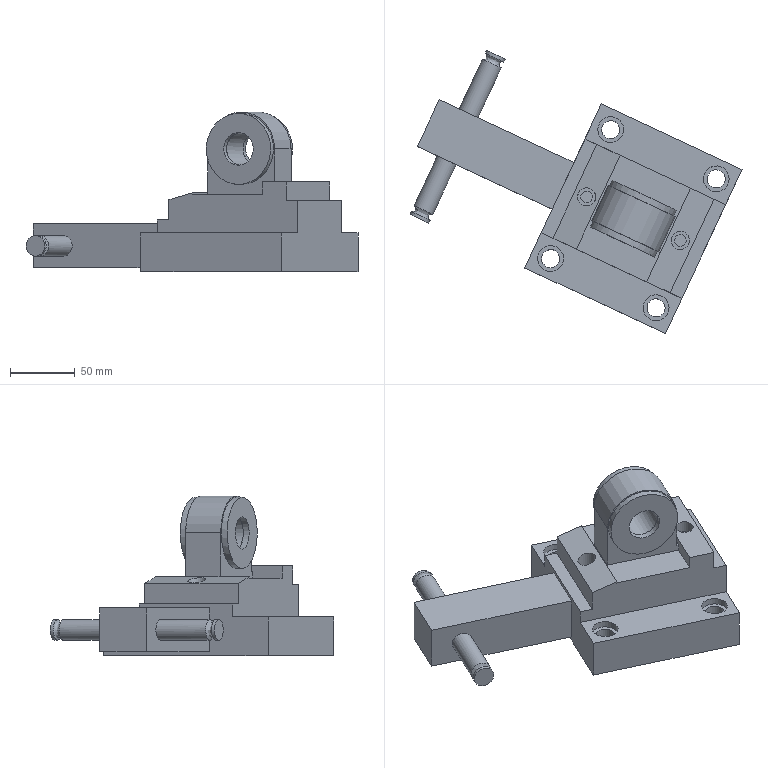Part | NX | features .3 ( *SOL6 - WSP HPSL15-R -  ) 2 | 1 solid | 70 faces | box 256.742 x 219.014 x 123.5 mm | volume 1031540 mm3 | plane 44 | cylinder 24 | spline 2 | commonest cylinder face diameters 14 x6 16 x4 20 x4 9 x2 13 x2 25.2 x2